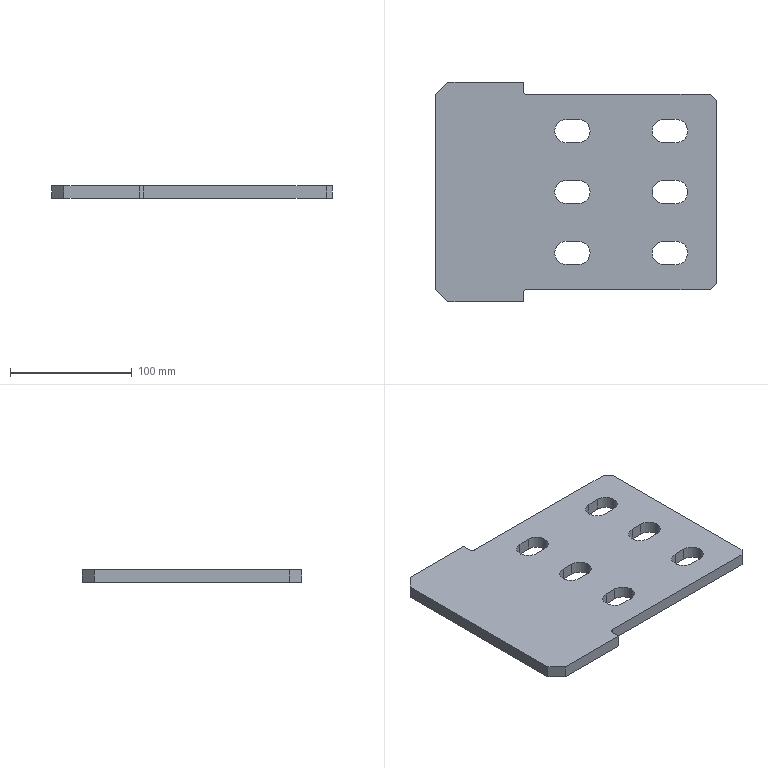Part | STEP file | 立柱腹Plate筋Plate-194×150-200 | 1 solid | 46 faces | box 230 x 180 x 10 mm | volume 352777 mm3 | plane 26 | cylinder 20 | commonest cylinder face diameters 19 x18 6 x2